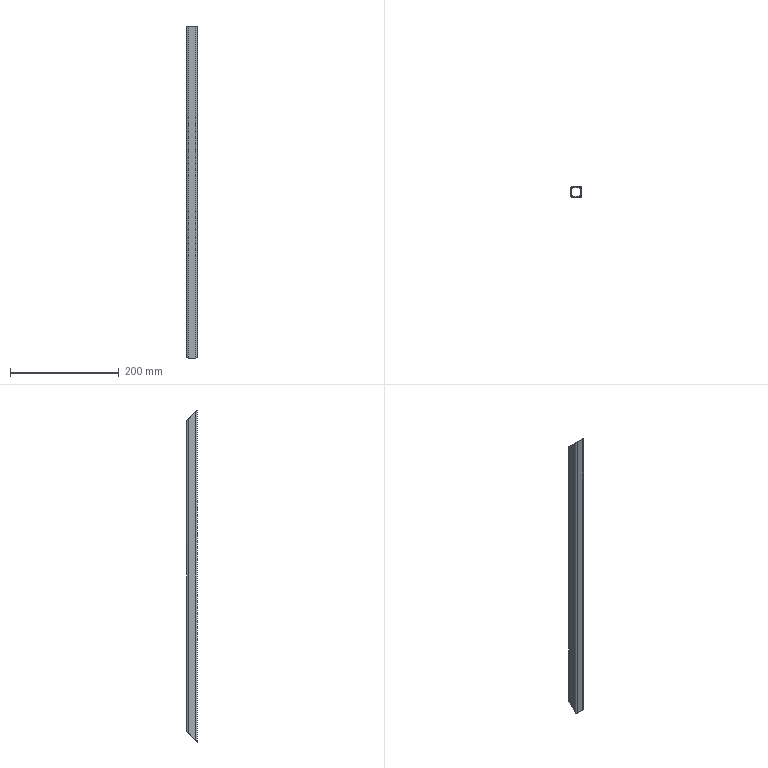Part | STEP file | DIN EN 10210-2 - 20 x 20 x 2 - 1000 | 1 solid | 18 faces | box 20 x 20 x 610 mm | volume 82428 mm3 | plane 10 | cylinder 8 | commonest cylinder face diameters 4 x4 6 x4